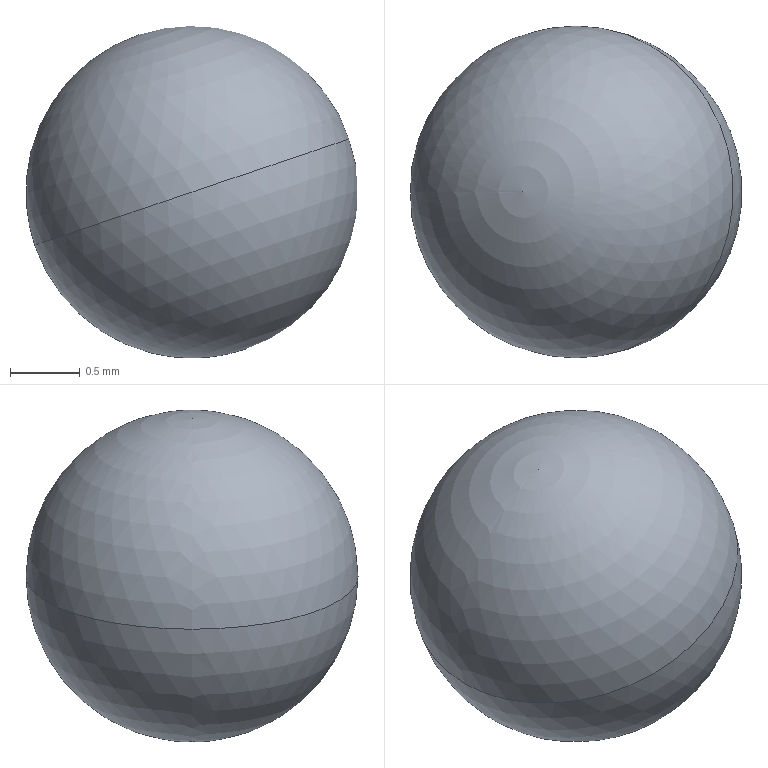Part | STEP file | 2026.6.15-Main Assembly图.sldasm-Part-179 | 1 solid | 2 faces | box 2.381 x 2.381 x 2.381 mm | volume 7.071 mm3 | sphere 2
STEP:
#1=CARTESIAN_POINT('',(-1477.791,1428.93,3247.943));
#2=VERTEX_POINT('',#1);
#3=CARTESIAN_POINT('',(-1477.791,1431.311,3247.943));
#4=VERTEX_POINT('',#3);
#5=CARTESIAN_POINT('',(-1477.791,1430.12,3247.943));
#6=DIRECTION('',(-0.3199,0.,0.9474));
#7=DIRECTION('',(0.,-1.,0.));
#8=AXIS2_PLACEMENT_3D('',#5,#6,#7);
#9=CIRCLE('',#8,1.191);
#10=EDGE_CURVE('',#2,#4,#9,.T.);
#11=ORIENTED_EDGE('',*,*,#10,.T.);
#12=CARTESIAN_POINT('',(-1477.791,1430.12,3247.943));
#13=DIRECTION('',(-0.3199,0.,0.9474));
#14=DIRECTION('',(0.,-1.,0.));
#15=AXIS2_PLACEMENT_3D('',#12,#13,#14);
#16=CIRCLE('',#15,1.191);
#17=EDGE_CURVE('',#4,#2,#16,.T.);
#18=ORIENTED_EDGE('',*,*,#17,.T.);
#19=EDGE_LOOP('',(#11,#18));
#20=FACE_OUTER_BOUND('',#19,.T.);
#21=CARTESIAN_POINT('',(-1477.791,1430.12,3247.943));
#22=DIRECTION('',(0.3199,0.,-0.9474));
#23=DIRECTION('',(-0.9474,0.,-0.3199));
#24=AXIS2_PLACEMENT_3D('',#21,#22,#23);
#25=SPHERICAL_SURFACE('',#24,1.191);
#26=ADVANCED_FACE('',(#20),#25,.T.);
#27=ORIENTED_EDGE('',*,*,#10,.F.);
#28=ORIENTED_EDGE('',*,*,#17,.F.);
#29=EDGE_LOOP('',(#27,#28));
#30=FACE_OUTER_BOUND('',#29,.T.);
#31=CARTESIAN_POINT('',(-1477.791,1430.12,3247.943));
#32=DIRECTION('',(0.3199,0.,-0.9474));
#33=DIRECTION('',(-0.9474,0.,-0.3199));
#34=AXIS2_PLACEMENT_3D('',#31,#32,#33);
#35=SPHERICAL_SURFACE('',#34,1.191);
#36=ADVANCED_FACE('',(#30),#35,.T.);
#37=CLOSED_SHELL('',(#26,#36));
#38=MANIFOLD_SOLID_BREP('',#37);
#39=CARTESIAN_POINT('',(0.,0.,0.));
#40=DIRECTION('',(0.,0.,1.));
#41=DIRECTION('',(1.,0.,0.));
#42=AXIS2_PLACEMENT_3D('',#39,#40,#41);
#43=(LENGTH_UNIT()NAMED_UNIT(*)SI_UNIT(.MILLI.,.METRE.));
#44=UNCERTAINTY_MEASURE_WITH_UNIT(LENGTH_MEASURE(0.00001),#43,'','');
#45=(NAMED_UNIT(*)PLANE_ANGLE_UNIT()SI_UNIT($,.RADIAN.));
#46=(NAMED_UNIT(*)SI_UNIT($,.STERADIAN.)SOLID_ANGLE_UNIT());
#47=(GEOMETRIC_REPRESENTATION_CONTEXT(3)GLOBAL_UNCERTAINTY_ASSIGNED_CONTEXT((#44))GLOBAL_UNIT_ASSIGNED_CONTEXT((#43,#45,#46))REPRESENTATION_CONTEXT('',''));
#48=ADVANCED_BREP_SHAPE_REPRESENTATION('',(#38,#42),#47);